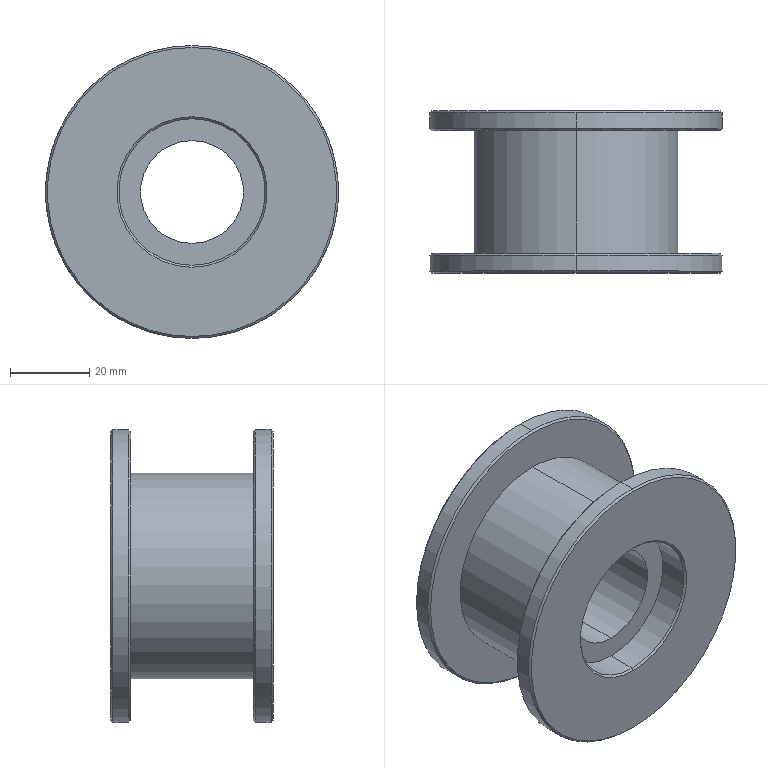Part | STEP file | adjusting belt tension wheel_SUS304 | 1 solid | 30 faces | box 74 x 41 x 74 mm | volume 78222 mm3 | cone 12 | cylinder 12 | plane 6 | commonest cylinder face diameters 37 x4 74 x4 26 x2 52 x2